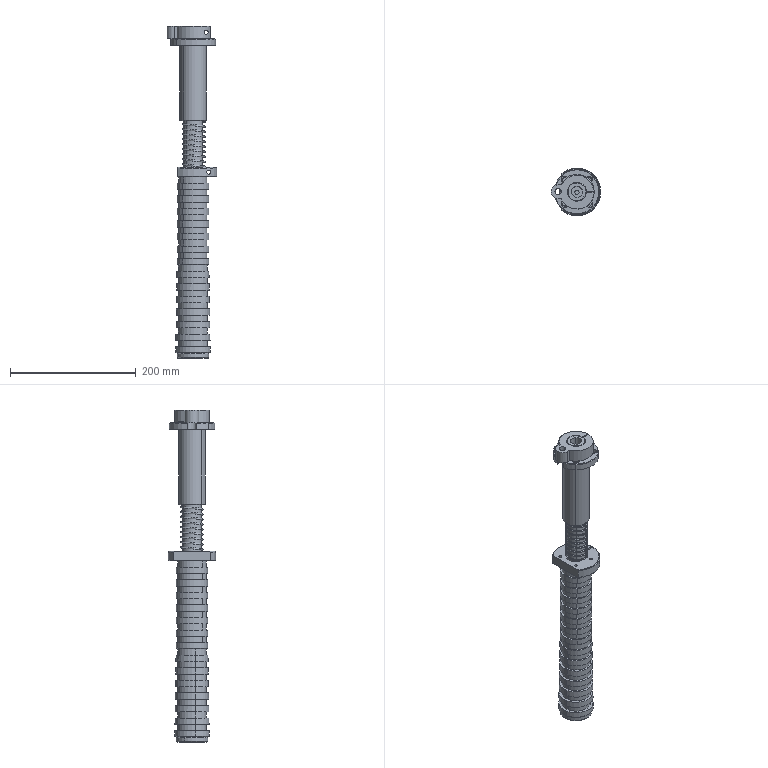Part | SolidWorks | features CompositeCurve 5 | 9 solids | 224 faces | box 78.987 x 76 x 528 mm | volume 773496 mm3 | cylinder 114 | plane 61 | cone 47 | spline 2 | commonest cylinder face diameters 50 x16 45 x14 46 x14 11 x13 30 x12 4.2 x8